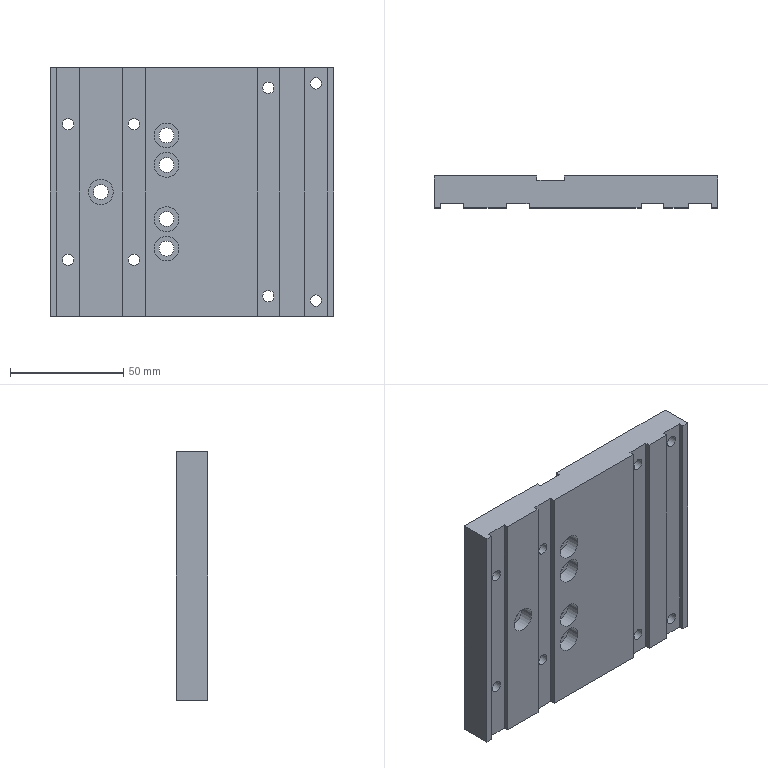NC program | NX | posted with a generic post | part box 125.5 x 14 x 110 mm
Whole program:
N10 G17 G21 G94 G90
(PLANAR_PROFILE , TOOL : D12)
N12 T00 M6
N14 G54
N16 G17 G0 G90 X69. Y0. S0 M3
N18 G43 Z20. H0
N20 Z-0.5
N22 G94 G1 X61. F250.
N24 Y-68.75
N26 X-61.
N28 Y68.75
N30 X61.
N32 Y0.
N34 X69.
N36 G0 Z-1.
N38 G1 X61.
N40 Y-68.75
N42 X-61.
N44 Y68.75
N46 X61.
N48 Y0.
N50 X69.
N52 G0 Z-1.5
N54 G1 X61.
N56 Y-68.75
N58 X-61.
N60 Y68.75
N62 X61.
N64 Y0.
N66 X69.
N68 G0 Z-2.
N70 G1 X61.
N72 Y-68.75
N74 X-61.
N76 Y68.75
N78 X61.
N80 Y0.
N82 X69.
N84 G0 Z-2.5
N86 G1 X61.
N88 Y-68.75
N90 X-61.
N92 Y68.75
N94 X61.
N96 Y0.
N98 X69.
N100 G0 Z-3.
N102 G1 X61.
N104 Y-68.75
N106 X-61.
N108 Y68.75
N110 X61.
N112 Y0.
N114 X69.
N116 G0 Z-3.5
N118 G1 X61.
N120 Y-68.75
N122 X-61.
N124 Y68.75
N126 X61.
N128 Y0.
N130 X69.
N132 G0 Z-4.
N134 G1 X61.
N136 Y-68.75
N138 X-61.
N140 Y68.75
N142 X61.
N144 Y0.
N146 X69.
N148 G0 Z-4.5
N150 G1 X61.
N152 Y-68.75
N154 X-61.
N156 Y68.75
N158 X61.
N160 Y0.
N162 X69.
N164 G0 Z-5.
N166 G1 X61.
N168 Y-68.75
N170 X-61.
N172 Y68.75
N174 X61.
N176 Y0.
N178 X69.
N180 G0 Z-5.5
N182 G1 X61.
N184 Y-68.75
N186 X-61.
N188 Y68.75
N190 X61.
N192 Y0.
N194 X69.
N196 G0 Z-6.
N198 G1 X61.
N200 Y-68.75
N202 X-61.
N204 Y68.75
N206 X61.
N208 Y0.
N210 X69.
N212 G0 Z-6.5
N214 G1 X61.
N216 Y-68.75
N218 X-61.
N220 Y68.75
N222 X61.
N224 Y0.
N226 X69.
N228 G0 Z-7.
N230 G1 X61.
N232 Y-68.75
N234 X-61.
N236 Y68.75
N238 X61.
N240 Y0.
N242 X69.
N244 G0 Z-7.5
N246 G1 X61.
N248 Y-68.75
N250 X-61.
N252 Y68.75
N254 X61.
N256 Y0.
N258 X69.
N260 G0 Z-8.
N262 G1 X61.
N264 Y-68.75
N266 X-61.
N268 Y68.75
N270 X61.
N272 Y0.
N274 X69.
N276 G0 Z-8.5
N278 G1 X61.
N280 Y-68.75
N282 X-61.
N284 Y68.75
N286 X61.
N288 Y0.
N290 X69.
N292 G0 Z-9.
N294 G1 X61.
N296 Y-68.75
N298 X-61.
N300 Y68.75
N302 X61.
N304 Y0.
N306 X69.
N308 G0 Z-9.5
N310 G1 X61.
N312 Y-68.75
N314 X-61.
N316 Y68.75
N318 X61.
N320 Y0.
N322 X69.
N324 G0 Z-10.
N326 G1 X61.
N328 Y-68.75
N330 X-61.
N332 Y68.75
N334 X61.
N336 Y0.
N338 X69.
N340 G0 Z-10.5
N342 G1 X61.
N344 Y-68.75
N346 X-61.
N348 Y68.75
N350 X61.
N352 Y0.
N354 X69.
N356 G0 Z-11.
N358 G1 X61.
N360 Y-68.75
N362 X-61.
N364 Y68.75
N366 X61.
N368 Y0.
N370 X69.
N372 G0 Z-11.5
N374 G1 X61.
N376 Y-68.75
N378 X-61.
N380 Y68.75
N382 X61.
N384 Y0.
N386 X69.
N388 G0 Z-12.
N390 G1 X61.
N392 Y-68.75
N394 X-61.
N396 Y68.75
N398 X61.
N400 Y0.
N402 X69.
N404 G0 Z-12.5
N406 G1 X61.
N408 Y-68.75
N410 X-61.
N412 Y68.75
N414 X61.
N416 Y0.
N418 X69.
N420 G0 Z-13.
N422 G1 X61.
N424 Y-68.75
N426 X-61.
N428 Y68.75
N430 X61.
N432 Y0.
N434 X69.
N436 G0 Z-13.5
N438 G1 X61.
N440 Y-68.75
N442 X-61.
N444 Y68.75
N446 X61.
N448 Y0.
N450 X69.
N452 G0 Z-14.
N454 G1 X61.
N456 Y-68.75
N458 X-61.
N460 Y68.75
N462 X61.
N464 Y0.
N466 X69.
N468 G0 Z20.
N470 M5
(FLOOR_WALL , TOOL : D8)
N472 M6
N474 G54
N476 G17 G0 G90 X62.15 Y-53.9 S0 M3
N478 G43 Z20. H0
N480 Z-0.4
N482 G94 G1 X55. F250.
N484 X-55.
N486 X-62.15
N488 Y-55.6
N490 X-55.
N492 X55.
N494 X62.15
N496 G0 Y-53.9 Z-0.8
N498 G1 X55.
N500 X-55.
N502 X-62.15
N504 Y-55.6
N506 X-55.
N508 X55.
N510 X62.15
N512 G0 Y-53.9 Z-1.2
N514 G1 X55.
N516 X-55.
N518 X-62.15
N520 Y-55.6
N522 X-55.
N524 X55.
N526 X62.15
N528 G0 Y-53.9 Z-1.6
N530 G1 X55.
N532 X-55.
N534 X-62.15
N536 Y-55.6
N538 X-55.
N540 X55.
N542 X62.15
N544 G0 Y-53.9 Z-2.
N546 G1 X55.
N548 X-55.
N550 X-62.15
N552 Y-55.6
N554 X-55.
N556 X55.
N558 X62.15
N560 G0 Z10.
N562 Y-24.9
N564 Z-0.4
N566 G1 X55.
N568 X-55.
N570 X-62.15
N572 Y-26.6
N574 X-55.
N576 X55.
N578 X62.15
N580 G0 Y-24.9 Z-0.8
N582 G1 X55.
N584 X-55.
N586 X-62.15
N588 Y-26.6
N590 X-55.
N592 X55.
N594 X62.15
N596 G0 Y-24.9 Z-1.2
N598 G1 X55.
N600 X-55.
N602 X-62.15
N604 Y-26.6
N606 X-55.
N608 X55.
N610 X62.15
N612 G0 Y-24.9 Z-1.6
N614 G1 X55.
N616 X-55.
N618 X-62.15
N620 Y-26.6
N622 X-55.
N624 X55.
N626 X62.15
N628 G0 Y-24.9 Z-2.
N630 G1 X55.
N632 X-55.
N634 X-62.15
N636 Y-26.6
N638 X-55.
N640 X55.
N642 X62.15
N644 G0 Z10.
N646 Y55.6
N648 Z-0.4
N650 G1 X55.
N652 X-55.
N654 X-62.15
N656 Y53.9
N658 X-55.
N660 X55.
N662 X62.15
N664 G0 Y55.6 Z-0.8
N666 G1 X55.
N668 X-55.
N670 X-62.15
N672 Y53.9
N674 X-55.
N676 X55.
N678 X62.15
N680 G0 Y55.6 Z-1.2
N682 G1 X55.
N684 X-55.
N686 X-62.15
N688 Y53.9
N690 X-55.
N692 X55.
N694 X62.15
N696 G0 Y55.6 Z-1.6
N698 G1 X55.
N700 X-55.
N702 X-62.15
N704 Y53.9
N706 X-55.
N708 X55.
N710 X62.15
N712 G0 Y55.6 Z-2.
N714 G1 X55.
N716 X-55.
N718 X-62.15
N720 Y53.9
N722 X-55.
N724 X55.
N726 X62.15
N728 G0 Z10.
N730 Y34.6
N732 Z-0.4
N734 G1 X55.
N736 X-55.
N738 X-62.15
N740 Y32.9
N742 X-55.
N744 X55.
N746 X62.15
N748 G0 Y34.6 Z-0.8
N750 G1 X55.
N752 X-55.
N754 X-62.15
N756 Y32.9
N758 X-55.
N760 X55.
N762 X62.15
N764 G0 Y34.6 Z-1.2
N766 G1 X55.
N768 X-55.
N770 X-62.15
N772 Y32.9
N774 X-55.
N776 X55.
N778 X62.15
N780 G0 Y34.6 Z-1.6
N782 G1 X55.
N784 X-55.
N786 X-62.15
N788 Y32.9
N790 X-55.
N792 X55.
N794 X62.15
N796 G0 Y34.6 Z-2.
N798 G1 X55.
N800 X-55.
N802 X-62.15
N804 Y32.9
N806 X-55.
N808 X55.
N810 X62.15
N812 G0 Z20.
(FLOOR_WALL_COPY , TOOL : D8)
N814 X62. Y-53.75
N816 Z-2.
N818 G1 X55.
N820 X-55.
N822 X-62.
N824 Y-55.75
N826 X-55.
N828 X55.
N830 X62.
N832 G0 Z10.
N834 Y-24.75
N836 Z-2.
N838 G1 X55.
N840 X-55.
N842 X-62.
N844 Y-26.75
N846 X-55.
N848 X55.
N850 X62.
N852 G0 Z10.
N854 Y55.75
N856 Z-2.
N858 G1 X55.
N860 X-55.
N862 X-62.
N864 Y53.75
N866 X-55.
N868 X55.
N870 X62.
N872 G0 Z10.
N874 Y34.75
N876 Z-2.
N878 G1 X55.
N880 X-55.
N882 X-62.
N884 Y32.75
N886 X-55.
N888 X55.
N890 X62.
N892 G0 Z20.
(SPOT_DRILLING , TOOL : D8)
N894 X30. Y-54.75
N896 G82 G99 Z0. P200 R3.
N898 X-30.
N900 X0. Y-40.25
N902 X30. Y-25.75
N904 X-30.
N906 X-25. Y-11.25
N908 X-12.
N910 X12.
N912 X25.
N914 X46. Y33.75
N916 X48. Y54.75
N918 X-48.
N920 X-46. Y33.75
N922 G80
N924 G0 X-46. Y33.75 Z20.
N926 M5
(HOLE_MILLING , TOOL : D6)
N928 M6
N930 G54
N932 G17 G0 G90 X0. Y-40.25 S0 M3
N934 G43 Z20. H0
N936 Z3.375
N938 G94 G3 X0. Y-42.6 Z3. I0. J-1.175 F250.
N940 X0. Y-42.6 Z1.5 I0. J2.35
N942 X0. Y-42.6 Z0. I0. J2.35
N944 X0. Y-42.6 Z-1.5 I0. J2.35
N946 X0. Y-42.6 Z-3. I0. J2.35
N948 X0. Y-42.6 Z-4.5 I0. J2.35
N950 X0. Y-42.6 Z-6. I0. J2.35
N952 X2.35 Y-40.25 R2.35
N954 X0. Y-42.6 R-2.35
N956 X0. Y-40.25 Z-5.25 I0. J1.175
N958 G0 Z20.
N960 X12. Y-11.25
N962 Z3.375
N964 G3 X12. Y-13.6 Z3. I0. J-1.175
N966 X12. Y-13.6 Z1.5 I0. J2.35
N968 X12. Y-13.6 Z0. I0. J2.35
N970 X12. Y-13.6 Z-1.5 I0. J2.35
N972 X12. Y-13.6 Z-3. I0. J2.35
N974 X12. Y-13.6 Z-4.5 I0. J2.35
N976 X12. Y-13.6 Z-6. I0. J2.35
N978 X14.35 Y-11.25 R2.35
N980 X12. Y-13.6 R-2.35
N982 X12. Y-11.25 Z-5.25 I0. J1.175
N984 G0 Z20.
N986 X-12.
N988 Z3.375
N990 G3 X-12. Y-13.6 Z3. I0. J-1.175
N992 X-12. Y-13.6 Z1.5 I0. J2.35
N994 X-12. Y-13.6 Z0. I0. J2.35
N996 X-12. Y-13.6 Z-1.5 I0. J2.35
N998 X-12. Y-13.6 Z-3. I0. J2.35
N1000 X-12. Y-13.6 Z-4.5 I0. J2.35
N1002 X-12. Y-13.6 Z-6. I0. J2.35
N1004 X-9.65 Y-11.25 R2.35
N1006 X-12. Y-13.6 R-2.35
N1008 X-12. Y-11.25 Z-5.25 I0. J1.175
N1010 G0 Z20.
N1012 X25.
N1014 Z3.375
N1016 G3 X25. Y-13.6 Z3. I0. J-1.175
N1018 X25. Y-13.6 Z1.5 I0. J2.35
N1020 X25. Y-13.6 Z0. I0. J2.35
N1022 X25. Y-13.6 Z-1.5 I0. J2.35
N1024 X25. Y-13.6 Z-3. I0. J2.35
N1026 X25. Y-13.6 Z-4.5 I0. J2.35
N1028 X25. Y-13.6 Z-6. I0. J2.35
N1030 X27.35 Y-11.25 R2.35
N1032 X25. Y-13.6 R-2.35
N1034 X25. Y-11.25 Z-5.25 I0. J1.175
N1036 G0 Z20.
N1038 X-25.
N1040 Z3.375
N1042 G3 X-25. Y-13.6 Z3. I0. J-1.175
N1044 X-25. Y-13.6 Z1.5 I0. J2.35
N1046 X-25. Y-13.6 Z0. I0. J2.35
N1048 X-25. Y-13.6 Z-1.5 I0. J2.35
N1050 X-25. Y-13.6 Z-3. I0. J2.35
N1052 X-25. Y-13.6 Z-4.5 I0. J2.35
N1054 X-25. Y-13.6 Z-6. I0. J2.35
N1056 X-22.65 Y-11.25 R2.35
N1058 X-25. Y-13.6 R-2.35
N1060 X-25. Y-11.25 Z-5.25 I0. J1.175
N1062 G0 Z20.
N1064 M5
N1066 M2